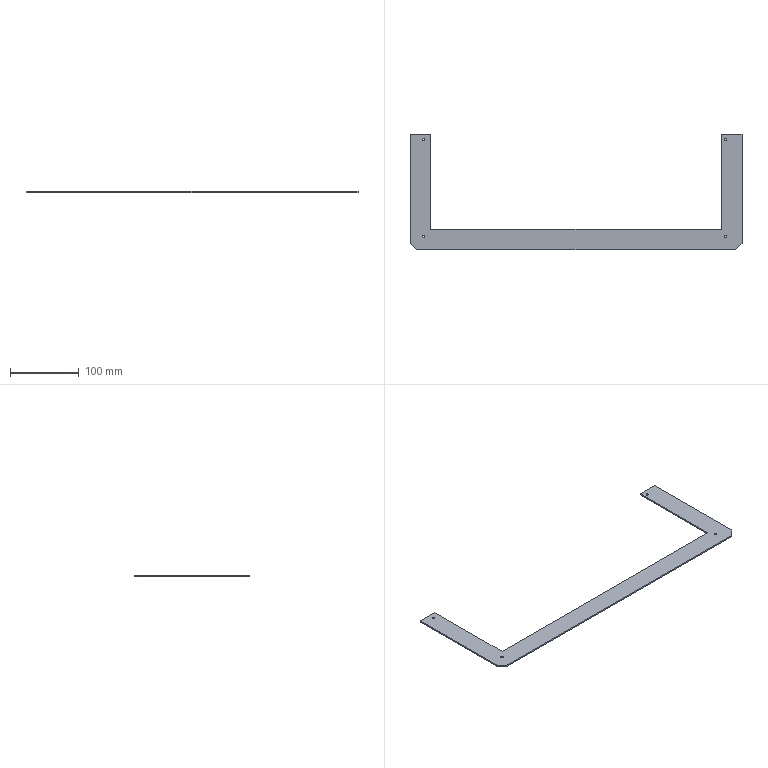Part | STEP file | Control Box Upper 3 | 1 solid | 20 faces | box 482 x 168.4 x 2 mm | volume 45264 mm3 | plane 12 | cylinder 8 | commonest cylinder face diameters 3.2 x8
STEP:
#1=CARTESIAN_POINT('',(31.6,-37.254,-2.));
#2=VERTEX_POINT('',#1);
#3=CARTESIAN_POINT('',(28.4,-37.254,-2.));
#4=VERTEX_POINT('',#3);
#5=CARTESIAN_POINT('',(30.,-37.254,-2.));
#6=DIRECTION('',(0.,0.,-1.));
#7=DIRECTION('',(1.,0.,0.));
#8=AXIS2_PLACEMENT_3D('',#5,#6,#7);
#9=CIRCLE('',#8,1.6);
#10=EDGE_CURVE('',#2,#4,#9,.T.);
#11=ORIENTED_EDGE('',*,*,#10,.T.);
#12=CARTESIAN_POINT('',(28.4,-37.254,0.));
#13=VERTEX_POINT('',#12);
#14=CARTESIAN_POINT('',(28.4,-37.254,-2.));
#15=DIRECTION('',(0.,0.,1.));
#16=VECTOR('',#15,1000.);
#17=LINE('',#14,#16);
#18=EDGE_CURVE('',#4,#13,#17,.T.);
#19=ORIENTED_EDGE('',*,*,#18,.T.);
#20=CARTESIAN_POINT('',(31.6,-37.254,0.));
#21=VERTEX_POINT('',#20);
#22=CARTESIAN_POINT('',(30.,-37.254,0.));
#23=DIRECTION('',(0.,0.,-1.));
#24=DIRECTION('',(1.,0.,0.));
#25=AXIS2_PLACEMENT_3D('',#22,#23,#24);
#26=CIRCLE('',#25,1.6);
#27=EDGE_CURVE('',#21,#13,#26,.T.);
#28=ORIENTED_EDGE('',*,*,#27,.F.);
#29=CARTESIAN_POINT('',(31.6,-37.254,-2.));
#30=DIRECTION('',(0.,0.,1.));
#31=VECTOR('',#30,1000.);
#32=LINE('',#29,#31);
#33=EDGE_CURVE('',#2,#21,#32,.T.);
#34=ORIENTED_EDGE('',*,*,#33,.F.);
#35=EDGE_LOOP('',(#11,#19,#28,#34));
#36=FACE_OUTER_BOUND('',#35,.T.);
#37=CARTESIAN_POINT('',(30.,-37.254,-2.));
#38=DIRECTION('',(0.,0.,1.));
#39=DIRECTION('',(1.,0.,0.));
#40=AXIS2_PLACEMENT_3D('',#37,#38,#39);
#41=CYLINDRICAL_SURFACE('',#40,1.6);
#42=ADVANCED_FACE('',(#36),#41,.F.);
#43=CARTESIAN_POINT('',(31.6,102.746,-2.));
#44=VERTEX_POINT('',#43);
#45=CARTESIAN_POINT('',(28.4,102.746,-2.));
#46=VERTEX_POINT('',#45);
#47=CARTESIAN_POINT('',(30.,102.746,-2.));
#48=DIRECTION('',(0.,0.,-1.));
#49=DIRECTION('',(1.,0.,0.));
#50=AXIS2_PLACEMENT_3D('',#47,#48,#49);
#51=CIRCLE('',#50,1.6);
#52=EDGE_CURVE('',#44,#46,#51,.T.);
#53=ORIENTED_EDGE('',*,*,#52,.T.);
#54=CARTESIAN_POINT('',(28.4,102.746,0.));
#55=VERTEX_POINT('',#54);
#56=CARTESIAN_POINT('',(28.4,102.746,-2.));
#57=DIRECTION('',(0.,0.,1.));
#58=VECTOR('',#57,1000.);
#59=LINE('',#56,#58);
#60=EDGE_CURVE('',#46,#55,#59,.T.);
#61=ORIENTED_EDGE('',*,*,#60,.T.);
#62=CARTESIAN_POINT('',(31.6,102.746,0.));
#63=VERTEX_POINT('',#62);
#64=CARTESIAN_POINT('',(30.,102.746,0.));
#65=DIRECTION('',(0.,0.,-1.));
#66=DIRECTION('',(1.,0.,0.));
#67=AXIS2_PLACEMENT_3D('',#64,#65,#66);
#68=CIRCLE('',#67,1.6);
#69=EDGE_CURVE('',#63,#55,#68,.T.);
#70=ORIENTED_EDGE('',*,*,#69,.F.);
#71=CARTESIAN_POINT('',(31.6,102.746,-2.));
#72=DIRECTION('',(0.,0.,1.));
#73=VECTOR('',#72,1000.);
#74=LINE('',#71,#73);
#75=EDGE_CURVE('',#44,#63,#74,.T.);
#76=ORIENTED_EDGE('',*,*,#75,.F.);
#77=EDGE_LOOP('',(#53,#61,#70,#76));
#78=FACE_OUTER_BOUND('',#77,.T.);
#79=CARTESIAN_POINT('',(30.,102.746,-2.));
#80=DIRECTION('',(0.,0.,1.));
#81=DIRECTION('',(1.,0.,0.));
#82=AXIS2_PLACEMENT_3D('',#79,#80,#81);
#83=CYLINDRICAL_SURFACE('',#82,1.6);
#84=ADVANCED_FACE('',(#78),#83,.F.);
#85=CARTESIAN_POINT('',(469.6,-37.254,-2.));
#86=VERTEX_POINT('',#85);
#87=CARTESIAN_POINT('',(466.4,-37.254,-2.));
#88=VERTEX_POINT('',#87);
#89=CARTESIAN_POINT('',(468.,-37.254,-2.));
#90=DIRECTION('',(0.,0.,-1.));
#91=DIRECTION('',(1.,0.,0.));
#92=AXIS2_PLACEMENT_3D('',#89,#90,#91);
#93=CIRCLE('',#92,1.6);
#94=EDGE_CURVE('',#86,#88,#93,.T.);
#95=ORIENTED_EDGE('',*,*,#94,.T.);
#96=CARTESIAN_POINT('',(466.4,-37.254,0.));
#97=VERTEX_POINT('',#96);
#98=CARTESIAN_POINT('',(466.4,-37.254,-2.));
#99=DIRECTION('',(0.,0.,1.));
#100=VECTOR('',#99,1000.);
#101=LINE('',#98,#100);
#102=EDGE_CURVE('',#88,#97,#101,.T.);
#103=ORIENTED_EDGE('',*,*,#102,.T.);
#104=CARTESIAN_POINT('',(469.6,-37.254,0.));
#105=VERTEX_POINT('',#104);
#106=CARTESIAN_POINT('',(468.,-37.254,0.));
#107=DIRECTION('',(0.,0.,-1.));
#108=DIRECTION('',(1.,0.,0.));
#109=AXIS2_PLACEMENT_3D('',#106,#107,#108);
#110=CIRCLE('',#109,1.6);
#111=EDGE_CURVE('',#105,#97,#110,.T.);
#112=ORIENTED_EDGE('',*,*,#111,.F.);
#113=CARTESIAN_POINT('',(469.6,-37.254,-2.));
#114=DIRECTION('',(0.,0.,1.));
#115=VECTOR('',#114,1000.);
#116=LINE('',#113,#115);
#117=EDGE_CURVE('',#86,#105,#116,.T.);
#118=ORIENTED_EDGE('',*,*,#117,.F.);
#119=EDGE_LOOP('',(#95,#103,#112,#118));
#120=FACE_OUTER_BOUND('',#119,.T.);
#121=CARTESIAN_POINT('',(468.,-37.254,-2.));
#122=DIRECTION('',(0.,0.,1.));
#123=DIRECTION('',(1.,0.,0.));
#124=AXIS2_PLACEMENT_3D('',#121,#122,#123);
#125=CYLINDRICAL_SURFACE('',#124,1.6);
#126=ADVANCED_FACE('',(#120),#125,.F.);
#127=CARTESIAN_POINT('',(469.6,102.746,-2.));
#128=VERTEX_POINT('',#127);
#129=CARTESIAN_POINT('',(466.4,102.746,-2.));
#130=VERTEX_POINT('',#129);
#131=CARTESIAN_POINT('',(468.,102.746,-2.));
#132=DIRECTION('',(0.,0.,-1.));
#133=DIRECTION('',(1.,0.,0.));
#134=AXIS2_PLACEMENT_3D('',#131,#132,#133);
#135=CIRCLE('',#134,1.6);
#136=EDGE_CURVE('',#128,#130,#135,.T.);
#137=ORIENTED_EDGE('',*,*,#136,.T.);
#138=CARTESIAN_POINT('',(466.4,102.746,0.));
#139=VERTEX_POINT('',#138);
#140=CARTESIAN_POINT('',(466.4,102.746,-2.));
#141=DIRECTION('',(0.,0.,1.));
#142=VECTOR('',#141,1000.);
#143=LINE('',#140,#142);
#144=EDGE_CURVE('',#130,#139,#143,.T.);
#145=ORIENTED_EDGE('',*,*,#144,.T.);
#146=CARTESIAN_POINT('',(469.6,102.746,0.));
#147=VERTEX_POINT('',#146);
#148=CARTESIAN_POINT('',(468.,102.746,0.));
#149=DIRECTION('',(0.,0.,-1.));
#150=DIRECTION('',(1.,0.,0.));
#151=AXIS2_PLACEMENT_3D('',#148,#149,#150);
#152=CIRCLE('',#151,1.6);
#153=EDGE_CURVE('',#147,#139,#152,.T.);
#154=ORIENTED_EDGE('',*,*,#153,.F.);
#155=CARTESIAN_POINT('',(469.6,102.746,-2.));
#156=DIRECTION('',(0.,0.,1.));
#157=VECTOR('',#156,1000.);
#158=LINE('',#155,#157);
#159=EDGE_CURVE('',#128,#147,#158,.T.);
#160=ORIENTED_EDGE('',*,*,#159,.F.);
#161=EDGE_LOOP('',(#137,#145,#154,#160));
#162=FACE_OUTER_BOUND('',#161,.T.);
#163=CARTESIAN_POINT('',(468.,102.746,-2.));
#164=DIRECTION('',(0.,0.,1.));
#165=DIRECTION('',(1.,0.,0.));
#166=AXIS2_PLACEMENT_3D('',#163,#164,#165);
#167=CYLINDRICAL_SURFACE('',#166,1.6);
#168=ADVANCED_FACE('',(#162),#167,.F.);
#169=CARTESIAN_POINT('',(10.,-47.254,-2.));
#170=VERTEX_POINT('',#169);
#171=CARTESIAN_POINT('',(20.,-57.254,-2.));
#172=VERTEX_POINT('',#171);
#173=CARTESIAN_POINT('',(10.,-47.254,-2.));
#174=DIRECTION('',(0.7071,-0.7071,0.));
#175=VECTOR('',#174,1000.);
#176=LINE('',#173,#175);
#177=EDGE_CURVE('',#170,#172,#176,.T.);
#178=ORIENTED_EDGE('',*,*,#177,.F.);
#179=CARTESIAN_POINT('',(10.,111.146,-2.));
#180=VERTEX_POINT('',#179);
#181=CARTESIAN_POINT('',(10.,0.,-2.));
#182=DIRECTION('',(0.,-1.,0.));
#183=VECTOR('',#182,1000.);
#184=LINE('',#181,#183);
#185=EDGE_CURVE('',#180,#170,#184,.T.);
#186=ORIENTED_EDGE('',*,*,#185,.F.);
#187=CARTESIAN_POINT('',(40.,111.146,-2.));
#188=VERTEX_POINT('',#187);
#189=CARTESIAN_POINT('',(0.,111.146,-2.));
#190=DIRECTION('',(-1.,0.,0.));
#191=VECTOR('',#190,1000.);
#192=LINE('',#189,#191);
#193=EDGE_CURVE('',#188,#180,#192,.T.);
#194=ORIENTED_EDGE('',*,*,#193,.F.);
#195=CARTESIAN_POINT('',(40.,-27.254,-2.));
#196=VERTEX_POINT('',#195);
#197=CARTESIAN_POINT('',(40.,0.,-2.));
#198=DIRECTION('',(0.,1.,0.));
#199=VECTOR('',#198,1000.);
#200=LINE('',#197,#199);
#201=EDGE_CURVE('',#196,#188,#200,.T.);
#202=ORIENTED_EDGE('',*,*,#201,.F.);
#203=CARTESIAN_POINT('',(462.,-27.254,-2.));
#204=VERTEX_POINT('',#203);
#205=CARTESIAN_POINT('',(0.,-27.254,-2.));
#206=DIRECTION('',(-1.,0.,0.));
#207=VECTOR('',#206,1000.);
#208=LINE('',#205,#207);
#209=EDGE_CURVE('',#204,#196,#208,.T.);
#210=ORIENTED_EDGE('',*,*,#209,.F.);
#211=CARTESIAN_POINT('',(462.,111.146,-2.));
#212=VERTEX_POINT('',#211);
#213=CARTESIAN_POINT('',(462.,0.,-2.));
#214=DIRECTION('',(0.,-1.,0.));
#215=VECTOR('',#214,1000.);
#216=LINE('',#213,#215);
#217=EDGE_CURVE('',#212,#204,#216,.T.);
#218=ORIENTED_EDGE('',*,*,#217,.F.);
#219=CARTESIAN_POINT('',(492.,111.146,-2.));
#220=VERTEX_POINT('',#219);
#221=CARTESIAN_POINT('',(0.,111.146,-2.));
#222=DIRECTION('',(-1.,0.,0.));
#223=VECTOR('',#222,1000.);
#224=LINE('',#221,#223);
#225=EDGE_CURVE('',#220,#212,#224,.T.);
#226=ORIENTED_EDGE('',*,*,#225,.F.);
#227=CARTESIAN_POINT('',(492.,-47.254,-2.));
#228=VERTEX_POINT('',#227);
#229=CARTESIAN_POINT('',(492.,0.,-2.));
#230=DIRECTION('',(0.,1.,0.));
#231=VECTOR('',#230,1000.);
#232=LINE('',#229,#231);
#233=EDGE_CURVE('',#228,#220,#232,.T.);
#234=ORIENTED_EDGE('',*,*,#233,.F.);
#235=CARTESIAN_POINT('',(482.,-57.254,-2.));
#236=VERTEX_POINT('',#235);
#237=CARTESIAN_POINT('',(482.,-57.254,-2.));
#238=DIRECTION('',(0.7071,0.7071,0.));
#239=VECTOR('',#238,1000.);
#240=LINE('',#237,#239);
#241=EDGE_CURVE('',#236,#228,#240,.T.);
#242=ORIENTED_EDGE('',*,*,#241,.F.);
#243=CARTESIAN_POINT('',(0.,-57.254,-2.));
#244=DIRECTION('',(1.,0.,0.));
#245=VECTOR('',#244,1000.);
#246=LINE('',#243,#245);
#247=EDGE_CURVE('',#172,#236,#246,.T.);
#248=ORIENTED_EDGE('',*,*,#247,.F.);
#249=EDGE_LOOP('',(#178,#186,#194,#202,#210,#218,#226,#234,#242,#248));
#250=FACE_OUTER_BOUND('',#249,.T.);
#251=ORIENTED_EDGE('',*,*,#10,.F.);
#252=CARTESIAN_POINT('',(30.,-37.254,-2.));
#253=DIRECTION('',(0.,0.,-1.));
#254=DIRECTION('',(1.,0.,0.));
#255=AXIS2_PLACEMENT_3D('',#252,#253,#254);
#256=CIRCLE('',#255,1.6);
#257=EDGE_CURVE('',#4,#2,#256,.T.);
#258=ORIENTED_EDGE('',*,*,#257,.F.);
#259=EDGE_LOOP('',(#251,#258));
#260=FACE_BOUND('',#259,.T.);
#261=ORIENTED_EDGE('',*,*,#52,.F.);
#262=CARTESIAN_POINT('',(30.,102.746,-2.));
#263=DIRECTION('',(0.,0.,-1.));
#264=DIRECTION('',(1.,0.,0.));
#265=AXIS2_PLACEMENT_3D('',#262,#263,#264);
#266=CIRCLE('',#265,1.6);
#267=EDGE_CURVE('',#46,#44,#266,.T.);
#268=ORIENTED_EDGE('',*,*,#267,.F.);
#269=EDGE_LOOP('',(#261,#268));
#270=FACE_BOUND('',#269,.T.);
#271=ORIENTED_EDGE('',*,*,#94,.F.);
#272=CARTESIAN_POINT('',(468.,-37.254,-2.));
#273=DIRECTION('',(0.,0.,-1.));
#274=DIRECTION('',(1.,0.,0.));
#275=AXIS2_PLACEMENT_3D('',#272,#273,#274);
#276=CIRCLE('',#275,1.6);
#277=EDGE_CURVE('',#88,#86,#276,.T.);
#278=ORIENTED_EDGE('',*,*,#277,.F.);
#279=EDGE_LOOP('',(#271,#278));
#280=FACE_BOUND('',#279,.T.);
#281=ORIENTED_EDGE('',*,*,#136,.F.);
#282=CARTESIAN_POINT('',(468.,102.746,-2.));
#283=DIRECTION('',(0.,0.,-1.));
#284=DIRECTION('',(1.,0.,0.));
#285=AXIS2_PLACEMENT_3D('',#282,#283,#284);
#286=CIRCLE('',#285,1.6);
#287=EDGE_CURVE('',#130,#128,#286,.T.);
#288=ORIENTED_EDGE('',*,*,#287,.F.);
#289=EDGE_LOOP('',(#281,#288));
#290=FACE_BOUND('',#289,.T.);
#291=CARTESIAN_POINT('',(0.,0.,-2.));
#292=DIRECTION('',(0.,0.,1.));
#293=DIRECTION('',(1.,0.,0.));
#294=AXIS2_PLACEMENT_3D('',#291,#292,#293);
#295=PLANE('',#294);
#296=ADVANCED_FACE('',(#250,#260,#270,#280,#290),#295,.F.);
#297=ORIENTED_EDGE('',*,*,#247,.T.);
#298=CARTESIAN_POINT('',(482.,-57.254,0.));
#299=VERTEX_POINT('',#298);
#300=CARTESIAN_POINT('',(482.,-57.254,-2.));
#301=DIRECTION('',(0.,0.,1.));
#302=VECTOR('',#301,1000.);
#303=LINE('',#300,#302);
#304=EDGE_CURVE('',#236,#299,#303,.T.);
#305=ORIENTED_EDGE('',*,*,#304,.T.);
#306=CARTESIAN_POINT('',(20.,-57.254,0.));
#307=VERTEX_POINT('',#306);
#308=CARTESIAN_POINT('',(10.,-57.254,0.));
#309=DIRECTION('',(-1.,0.,0.));
#310=VECTOR('',#309,1000.);
#311=LINE('',#308,#310);
#312=EDGE_CURVE('',#299,#307,#311,.T.);
#313=ORIENTED_EDGE('',*,*,#312,.T.);
#314=CARTESIAN_POINT('',(20.,-57.254,-2.));
#315=DIRECTION('',(0.,0.,-1.));
#316=VECTOR('',#315,1000.);
#317=LINE('',#314,#316);
#318=EDGE_CURVE('',#307,#172,#317,.T.);
#319=ORIENTED_EDGE('',*,*,#318,.T.);
#320=EDGE_LOOP('',(#297,#305,#313,#319));
#321=FACE_OUTER_BOUND('',#320,.T.);
#322=CARTESIAN_POINT('',(10.,-57.254,-2.));
#323=DIRECTION('',(0.,-1.,0.));
#324=DIRECTION('',(0.,0.,-1.));
#325=AXIS2_PLACEMENT_3D('',#322,#323,#324);
#326=PLANE('',#325);
#327=ADVANCED_FACE('',(#321),#326,.T.);
#328=ORIENTED_EDGE('',*,*,#318,.F.);
#329=CARTESIAN_POINT('',(10.,-47.254,0.));
#330=VERTEX_POINT('',#329);
#331=CARTESIAN_POINT('',(10.,-47.254,0.));
#332=DIRECTION('',(0.7071,-0.7071,0.));
#333=VECTOR('',#332,1000.);
#334=LINE('',#331,#333);
#335=EDGE_CURVE('',#330,#307,#334,.T.);
#336=ORIENTED_EDGE('',*,*,#335,.F.);
#337=CARTESIAN_POINT('',(10.,-47.254,-2.));
#338=DIRECTION('',(0.,0.,1.));
#339=VECTOR('',#338,1000.);
#340=LINE('',#337,#339);
#341=EDGE_CURVE('',#170,#330,#340,.T.);
#342=ORIENTED_EDGE('',*,*,#341,.F.);
#343=ORIENTED_EDGE('',*,*,#177,.T.);
#344=EDGE_LOOP('',(#328,#336,#342,#343));
#345=FACE_OUTER_BOUND('',#344,.T.);
#346=CARTESIAN_POINT('',(10.,-47.254,-2.));
#347=DIRECTION('',(0.7071,0.7071,0.));
#348=DIRECTION('',(-0.7071,0.7071,0.));
#349=AXIS2_PLACEMENT_3D('',#346,#347,#348);
#350=PLANE('',#349);
#351=ADVANCED_FACE('',(#345),#350,.F.);
#352=CARTESIAN_POINT('',(10.,111.146,0.));
#353=VERTEX_POINT('',#352);
#354=CARTESIAN_POINT('',(10.,112.746,0.));
#355=DIRECTION('',(0.,1.,0.));
#356=VECTOR('',#355,1000.);
#357=LINE('',#354,#356);
#358=EDGE_CURVE('',#330,#353,#357,.T.);
#359=ORIENTED_EDGE('',*,*,#358,.T.);
#360=CARTESIAN_POINT('',(10.,111.146,-2.));
#361=DIRECTION('',(0.,0.,-1.));
#362=VECTOR('',#361,1000.);
#363=LINE('',#360,#362);
#364=EDGE_CURVE('',#353,#180,#363,.T.);
#365=ORIENTED_EDGE('',*,*,#364,.T.);
#366=ORIENTED_EDGE('',*,*,#185,.T.);
#367=ORIENTED_EDGE('',*,*,#341,.T.);
#368=EDGE_LOOP('',(#359,#365,#366,#367));
#369=FACE_OUTER_BOUND('',#368,.T.);
#370=CARTESIAN_POINT('',(10.,112.746,-2.));
#371=DIRECTION('',(-1.,0.,0.));
#372=DIRECTION('',(0.,-1.,0.));
#373=AXIS2_PLACEMENT_3D('',#370,#371,#372);
#374=PLANE('',#373);
#375=ADVANCED_FACE('',(#369),#374,.T.);
#376=CARTESIAN_POINT('',(40.,111.146,0.));
#377=VERTEX_POINT('',#376);
#378=CARTESIAN_POINT('',(10.,111.146,0.));
#379=DIRECTION('',(-1.,0.,0.));
#380=VECTOR('',#379,1000.);
#381=LINE('',#378,#380);
#382=EDGE_CURVE('',#377,#353,#381,.T.);
#383=ORIENTED_EDGE('',*,*,#382,.F.);
#384=CARTESIAN_POINT('',(40.,111.146,-10.));
#385=DIRECTION('',(0.,0.,1.));
#386=VECTOR('',#385,1000.);
#387=LINE('',#384,#386);
#388=EDGE_CURVE('',#188,#377,#387,.T.);
#389=ORIENTED_EDGE('',*,*,#388,.F.);
#390=ORIENTED_EDGE('',*,*,#193,.T.);
#391=ORIENTED_EDGE('',*,*,#364,.F.);
#392=EDGE_LOOP('',(#383,#389,#390,#391));
#393=FACE_OUTER_BOUND('',#392,.T.);
#394=CARTESIAN_POINT('',(10.,111.146,-10.));
#395=DIRECTION('',(0.,-1.,0.));
#396=DIRECTION('',(0.,0.,-1.));
#397=AXIS2_PLACEMENT_3D('',#394,#395,#396);
#398=PLANE('',#397);
#399=ADVANCED_FACE('',(#393),#398,.F.);
#400=CARTESIAN_POINT('',(40.,-27.254,0.));
#401=VERTEX_POINT('',#400);
#402=CARTESIAN_POINT('',(40.,-27.254,-2.));
#403=DIRECTION('',(0.,0.,-1.));
#404=VECTOR('',#403,1000.);
#405=LINE('',#402,#404);
#406=EDGE_CURVE('',#401,#196,#405,.T.);
#407=ORIENTED_EDGE('',*,*,#406,.T.);
#408=ORIENTED_EDGE('',*,*,#201,.T.);
#409=ORIENTED_EDGE('',*,*,#388,.T.);
#410=CARTESIAN_POINT('',(40.,-27.254,0.));
#411=DIRECTION('',(0.,-1.,0.));
#412=VECTOR('',#411,1000.);
#413=LINE('',#410,#412);
#414=EDGE_CURVE('',#377,#401,#413,.T.);
#415=ORIENTED_EDGE('',*,*,#414,.T.);
#416=EDGE_LOOP('',(#407,#408,#409,#415));
#417=FACE_OUTER_BOUND('',#416,.T.);
#418=CARTESIAN_POINT('',(40.,-27.254,-2.));
#419=DIRECTION('',(1.,0.,0.));
#420=DIRECTION('',(0.,1.,0.));
#421=AXIS2_PLACEMENT_3D('',#418,#419,#420);
#422=PLANE('',#421);
#423=ADVANCED_FACE('',(#417),#422,.T.);
#424=ORIENTED_EDGE('',*,*,#209,.T.);
#425=ORIENTED_EDGE('',*,*,#406,.F.);
#426=CARTESIAN_POINT('',(462.,-27.254,0.));
#427=VERTEX_POINT('',#426);
#428=CARTESIAN_POINT('',(462.,-27.254,0.));
#429=DIRECTION('',(1.,0.,0.));
#430=VECTOR('',#429,1000.);
#431=LINE('',#428,#430);
#432=EDGE_CURVE('',#401,#427,#431,.T.);
#433=ORIENTED_EDGE('',*,*,#432,.T.);
#434=CARTESIAN_POINT('',(462.,-27.254,-2.));
#435=DIRECTION('',(0.,0.,-1.));
#436=VECTOR('',#435,1000.);
#437=LINE('',#434,#436);
#438=EDGE_CURVE('',#427,#204,#437,.T.);
#439=ORIENTED_EDGE('',*,*,#438,.T.);
#440=EDGE_LOOP('',(#424,#425,#433,#439));
#441=FACE_OUTER_BOUND('',#440,.T.);
#442=CARTESIAN_POINT('',(462.,-27.254,-2.));
#443=DIRECTION('',(0.,1.,0.));
#444=DIRECTION('',(0.,0.,1.));
#445=AXIS2_PLACEMENT_3D('',#442,#443,#444);
#446=PLANE('',#445);
#447=ADVANCED_FACE('',(#441),#446,.T.);
#448=ORIENTED_EDGE('',*,*,#438,.F.);
#449=CARTESIAN_POINT('',(462.,111.146,0.));
#450=VERTEX_POINT('',#449);
#451=CARTESIAN_POINT('',(462.,112.746,0.));
#452=DIRECTION('',(0.,1.,0.));
#453=VECTOR('',#452,1000.);
#454=LINE('',#451,#453);
#455=EDGE_CURVE('',#427,#450,#454,.T.);
#456=ORIENTED_EDGE('',*,*,#455,.T.);
#457=CARTESIAN_POINT('',(462.,111.146,-2.));
#458=DIRECTION('',(0.,0.,-1.));
#459=VECTOR('',#458,1000.);
#460=LINE('',#457,#459);
#461=EDGE_CURVE('',#450,#212,#460,.T.);
#462=ORIENTED_EDGE('',*,*,#461,.T.);
#463=ORIENTED_EDGE('',*,*,#217,.T.);
#464=EDGE_LOOP('',(#448,#456,#462,#463));
#465=FACE_OUTER_BOUND('',#464,.T.);
#466=CARTESIAN_POINT('',(462.,112.746,-2.));
#467=DIRECTION('',(-1.,0.,0.));
#468=DIRECTION('',(0.,0.,1.));
#469=AXIS2_PLACEMENT_3D('',#466,#467,#468);
#470=PLANE('',#469);
#471=ADVANCED_FACE('',(#465),#470,.T.);
#472=CARTESIAN_POINT('',(492.,111.146,0.));
#473=VERTEX_POINT('',#472);
#474=CARTESIAN_POINT('',(462.,111.146,0.));
#475=DIRECTION('',(-1.,0.,0.));
#476=VECTOR('',#475,1000.);
#477=LINE('',#474,#476);
#478=EDGE_CURVE('',#473,#450,#477,.T.);
#479=ORIENTED_EDGE('',*,*,#478,.F.);
#480=CARTESIAN_POINT('',(492.,111.146,-10.));
#481=DIRECTION('',(0.,0.,1.));
#482=VECTOR('',#481,1000.);
#483=LINE('',#480,#482);
#484=EDGE_CURVE('',#220,#473,#483,.T.);
#485=ORIENTED_EDGE('',*,*,#484,.F.);
#486=ORIENTED_EDGE('',*,*,#225,.T.);
#487=ORIENTED_EDGE('',*,*,#461,.F.);
#488=EDGE_LOOP('',(#479,#485,#486,#487));
#489=FACE_OUTER_BOUND('',#488,.T.);
#490=CARTESIAN_POINT('',(462.,111.146,-10.));
#491=DIRECTION('',(0.,-1.,0.));
#492=DIRECTION('',(0.,0.,-1.));
#493=AXIS2_PLACEMENT_3D('',#490,#491,#492);
#494=PLANE('',#493);
#495=ADVANCED_FACE('',(#489),#494,.F.);
#496=ORIENTED_EDGE('',*,*,#233,.T.);
#497=ORIENTED_EDGE('',*,*,#484,.T.);
#498=CARTESIAN_POINT('',(492.,-47.254,0.));
#499=VERTEX_POINT('',#498);
#500=CARTESIAN_POINT('',(492.,-57.254,0.));
#501=DIRECTION('',(0.,-1.,0.));
#502=VECTOR('',#501,1000.);
#503=LINE('',#500,#502);
#504=EDGE_CURVE('',#473,#499,#503,.T.);
#505=ORIENTED_EDGE('',*,*,#504,.T.);
#506=CARTESIAN_POINT('',(492.,-47.254,-2.));
#507=DIRECTION('',(0.,0.,-1.));
#508=VECTOR('',#507,1000.);
#509=LINE('',#506,#508);
#510=EDGE_CURVE('',#499,#228,#509,.T.);
#511=ORIENTED_EDGE('',*,*,#510,.T.);
#512=EDGE_LOOP('',(#496,#497,#505,#511));
#513=FACE_OUTER_BOUND('',#512,.T.);
#514=CARTESIAN_POINT('',(492.,-57.254,-2.));
#515=DIRECTION('',(1.,0.,0.));
#516=DIRECTION('',(0.,0.,-1.));
#517=AXIS2_PLACEMENT_3D('',#514,#515,#516);
#518=PLANE('',#517);
#519=ADVANCED_FACE('',(#513),#518,.T.);
#520=ORIENTED_EDGE('',*,*,#510,.F.);
#521=CARTESIAN_POINT('',(482.,-57.254,0.));
#522=DIRECTION('',(0.7071,0.7071,0.));
#523=VECTOR('',#522,1000.);
#524=LINE('',#521,#523);
#525=EDGE_CURVE('',#299,#499,#524,.T.);
#526=ORIENTED_EDGE('',*,*,#525,.F.);
#527=ORIENTED_EDGE('',*,*,#304,.F.);
#528=ORIENTED_EDGE('',*,*,#241,.T.);
#529=EDGE_LOOP('',(#520,#526,#527,#528));
#530=FACE_OUTER_BOUND('',#529,.T.);
#531=CARTESIAN_POINT('',(482.,-57.254,-2.));
#532=DIRECTION('',(-0.7071,0.7071,0.));
#533=DIRECTION('',(-0.7071,-0.7071,0.));
#534=AXIS2_PLACEMENT_3D('',#531,#532,#533);
#535=PLANE('',#534);
#536=ADVANCED_FACE('',(#530),#535,.F.);
#537=ORIENTED_EDGE('',*,*,#18,.F.);
#538=ORIENTED_EDGE('',*,*,#257,.T.);
#539=ORIENTED_EDGE('',*,*,#33,.T.);
#540=CARTESIAN_POINT('',(30.,-37.254,0.));
#541=DIRECTION('',(0.,0.,-1.));
#542=DIRECTION('',(1.,0.,0.));
#543=AXIS2_PLACEMENT_3D('',#540,#541,#542);
#544=CIRCLE('',#543,1.6);
#545=EDGE_CURVE('',#13,#21,#544,.T.);
#546=ORIENTED_EDGE('',*,*,#545,.F.);
#547=EDGE_LOOP('',(#537,#538,#539,#546));
#548=FACE_OUTER_BOUND('',#547,.T.);
#549=CARTESIAN_POINT('',(30.,-37.254,-2.));
#550=DIRECTION('',(0.,0.,1.));
#551=DIRECTION('',(1.,0.,0.));
#552=AXIS2_PLACEMENT_3D('',#549,#550,#551);
#553=CYLINDRICAL_SURFACE('',#552,1.6);
#554=ADVANCED_FACE('',(#548),#553,.F.);
#555=ORIENTED_EDGE('',*,*,#60,.F.);
#556=ORIENTED_EDGE('',*,*,#267,.T.);
#557=ORIENTED_EDGE('',*,*,#75,.T.);
#558=CARTESIAN_POINT('',(30.,102.746,0.));
#559=DIRECTION('',(0.,0.,-1.));
#560=DIRECTION('',(1.,0.,0.));
#561=AXIS2_PLACEMENT_3D('',#558,#559,#560);
#562=CIRCLE('',#561,1.6);
#563=EDGE_CURVE('',#55,#63,#562,.T.);
#564=ORIENTED_EDGE('',*,*,#563,.F.);
#565=EDGE_LOOP('',(#555,#556,#557,#564));
#566=FACE_OUTER_BOUND('',#565,.T.);
#567=CARTESIAN_POINT('',(30.,102.746,-2.));
#568=DIRECTION('',(0.,0.,1.));
#569=DIRECTION('',(1.,0.,0.));
#570=AXIS2_PLACEMENT_3D('',#567,#568,#569);
#571=CYLINDRICAL_SURFACE('',#570,1.6);
#572=ADVANCED_FACE('',(#566),#571,.F.);
#573=ORIENTED_EDGE('',*,*,#102,.F.);
#574=ORIENTED_EDGE('',*,*,#277,.T.);
#575=ORIENTED_EDGE('',*,*,#117,.T.);
#576=CARTESIAN_POINT('',(468.,-37.254,0.));
#577=DIRECTION('',(0.,0.,-1.));
#578=DIRECTION('',(1.,0.,0.));
#579=AXIS2_PLACEMENT_3D('',#576,#577,#578);
#580=CIRCLE('',#579,1.6);
#581=EDGE_CURVE('',#97,#105,#580,.T.);
#582=ORIENTED_EDGE('',*,*,#581,.F.);
#583=EDGE_LOOP('',(#573,#574,#575,#582));
#584=FACE_OUTER_BOUND('',#583,.T.);
#585=CARTESIAN_POINT('',(468.,-37.254,-2.));
#586=DIRECTION('',(0.,0.,1.));
#587=DIRECTION('',(1.,0.,0.));
#588=AXIS2_PLACEMENT_3D('',#585,#586,#587);
#589=CYLINDRICAL_SURFACE('',#588,1.6);
#590=ADVANCED_FACE('',(#584),#589,.F.);
#591=ORIENTED_EDGE('',*,*,#144,.F.);
#592=ORIENTED_EDGE('',*,*,#287,.T.);
#593=ORIENTED_EDGE('',*,*,#159,.T.);
#594=CARTESIAN_POINT('',(468.,102.746,0.));
#595=DIRECTION('',(0.,0.,-1.));
#596=DIRECTION('',(1.,0.,0.));
#597=AXIS2_PLACEMENT_3D('',#594,#595,#596);
#598=CIRCLE('',#597,1.6);
#599=EDGE_CURVE('',#139,#147,#598,.T.);
#600=ORIENTED_EDGE('',*,*,#599,.F.);
#601=EDGE_LOOP('',(#591,#592,#593,#600));
#602=FACE_OUTER_BOUND('',#601,.T.);
#603=CARTESIAN_POINT('',(468.,102.746,-2.));
#604=DIRECTION('',(0.,0.,1.));
#605=DIRECTION('',(1.,0.,0.));
#606=AXIS2_PLACEMENT_3D('',#603,#604,#605);
#607=CYLINDRICAL_SURFACE('',#606,1.6);
#608=ADVANCED_FACE('',(#602),#607,.F.);
#609=ORIENTED_EDGE('',*,*,#27,.T.);
#610=ORIENTED_EDGE('',*,*,#545,.T.);
#611=EDGE_LOOP('',(#609,#610));
#612=FACE_BOUND('',#611,.T.);
#613=ORIENTED_EDGE('',*,*,#69,.T.);
#614=ORIENTED_EDGE('',*,*,#563,.T.);
#615=EDGE_LOOP('',(#613,#614));
#616=FACE_BOUND('',#615,.T.);
#617=ORIENTED_EDGE('',*,*,#111,.T.);
#618=ORIENTED_EDGE('',*,*,#581,.T.);
#619=EDGE_LOOP('',(#617,#618));
#620=FACE_BOUND('',#619,.T.);
#621=ORIENTED_EDGE('',*,*,#153,.T.);
#622=ORIENTED_EDGE('',*,*,#599,.T.);
#623=EDGE_LOOP('',(#621,#622));
#624=FACE_BOUND('',#623,.T.);
#625=ORIENTED_EDGE('',*,*,#414,.F.);
#626=ORIENTED_EDGE('',*,*,#382,.T.);
#627=ORIENTED_EDGE('',*,*,#358,.F.);
#628=ORIENTED_EDGE('',*,*,#335,.T.);
#629=ORIENTED_EDGE('',*,*,#312,.F.);
#630=ORIENTED_EDGE('',*,*,#525,.T.);
#631=ORIENTED_EDGE('',*,*,#504,.F.);
#632=ORIENTED_EDGE('',*,*,#478,.T.);
#633=ORIENTED_EDGE('',*,*,#455,.F.);
#634=ORIENTED_EDGE('',*,*,#432,.F.);
#635=EDGE_LOOP('',(#625,#626,#627,#628,#629,#630,#631,#632,#633,#634));
#636=FACE_OUTER_BOUND('',#635,.T.);
#637=CARTESIAN_POINT('',(0.,0.,0.));
#638=DIRECTION('',(0.,0.,1.));
#639=DIRECTION('',(1.,0.,0.));
#640=AXIS2_PLACEMENT_3D('',#637,#638,#639);
#641=PLANE('',#640);
#642=ADVANCED_FACE('',(#612,#616,#620,#624,#636),#641,.T.);
#643=CLOSED_SHELL('',(#42,#84,#126,#168,#296,#327,#351,#375,#399,#423,#447,#471,#495,#519,#536,#554,#572,#590,#608,#642));
#644=MANIFOLD_SOLID_BREP('',#643);
#645=CARTESIAN_POINT('',(0.,0.,0.));
#646=DIRECTION('',(0.,0.,1.));
#647=DIRECTION('',(1.,0.,0.));
#648=AXIS2_PLACEMENT_3D('',#645,#646,#647);
#649=(LENGTH_UNIT()NAMED_UNIT(*)SI_UNIT(.MILLI.,.METRE.));
#650=UNCERTAINTY_MEASURE_WITH_UNIT(LENGTH_MEASURE(0.00001),#649,'','');
#651=(NAMED_UNIT(*)PLANE_ANGLE_UNIT()SI_UNIT($,.RADIAN.));
#652=(NAMED_UNIT(*)SI_UNIT($,.STERADIAN.)SOLID_ANGLE_UNIT());
#653=(GEOMETRIC_REPRESENTATION_CONTEXT(3)GLOBAL_UNCERTAINTY_ASSIGNED_CONTEXT((#650))GLOBAL_UNIT_ASSIGNED_CONTEXT((#649,#651,#652))REPRESENTATION_CONTEXT('',''));
#654=ADVANCED_BREP_SHAPE_REPRESENTATION('',(#644,#648),#653);